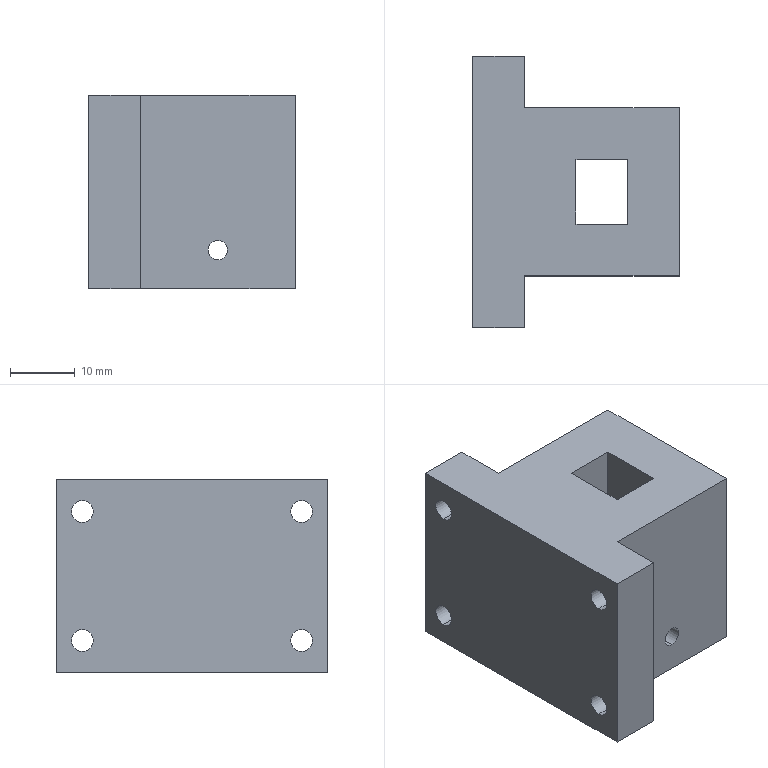Part | STEP file | X77b-01014 | 1 solid | 41 faces | box 32 x 42 x 30 mm | volume 25333 mm3 | cylinder 22 | plane 19 | commonest cylinder face diameters 3.4 x8 6 x8 3 x4 8 x2
STEP:
#1=CARTESIAN_POINT('',(-15.4,-53.814,28.));
#2=VERTEX_POINT('',#1);
#3=CARTESIAN_POINT('',(-15.4,-53.814,22.));
#4=VERTEX_POINT('',#3);
#5=CARTESIAN_POINT('',(-15.4,-53.814,25.));
#6=DIRECTION('',(1.,0.,0.));
#7=DIRECTION('',(0.,0.,-1.));
#8=AXIS2_PLACEMENT_3D('',#5,#6,#7);
#9=CIRCLE('',#8,3.);
#10=EDGE_CURVE('',#2,#4,#9,.T.);
#11=ORIENTED_EDGE('',*,*,#10,.F.);
#12=CARTESIAN_POINT('',(-12.,-53.814,28.));
#13=VERTEX_POINT('',#12);
#14=CARTESIAN_POINT('',(-12.,-53.814,28.));
#15=DIRECTION('',(1.,0.,0.));
#16=VECTOR('',#15,1000.);
#17=LINE('',#14,#16);
#18=EDGE_CURVE('',#2,#13,#17,.T.);
#19=ORIENTED_EDGE('',*,*,#18,.T.);
#20=CARTESIAN_POINT('',(-12.,-53.814,22.));
#21=VERTEX_POINT('',#20);
#22=CARTESIAN_POINT('',(-12.,-53.814,25.));
#23=DIRECTION('',(1.,0.,0.));
#24=DIRECTION('',(0.,0.,-1.));
#25=AXIS2_PLACEMENT_3D('',#22,#23,#24);
#26=CIRCLE('',#25,3.);
#27=EDGE_CURVE('',#13,#21,#26,.T.);
#28=ORIENTED_EDGE('',*,*,#27,.T.);
#29=CARTESIAN_POINT('',(-12.,-53.814,22.));
#30=DIRECTION('',(1.,0.,0.));
#31=VECTOR('',#30,1000.);
#32=LINE('',#29,#31);
#33=EDGE_CURVE('',#4,#21,#32,.T.);
#34=ORIENTED_EDGE('',*,*,#33,.F.);
#35=EDGE_LOOP('',(#11,#19,#28,#34));
#36=FACE_OUTER_BOUND('',#35,.T.);
#37=CARTESIAN_POINT('',(-12.,-53.814,25.));
#38=DIRECTION('',(1.,0.,0.));
#39=DIRECTION('',(0.,0.,-1.));
#40=AXIS2_PLACEMENT_3D('',#37,#38,#39);
#41=CYLINDRICAL_SURFACE('',#40,3.);
#42=ADVANCED_FACE('',(#36),#41,.F.);
#43=CARTESIAN_POINT('',(-20.,-53.814,26.7));
#44=VERTEX_POINT('',#43);
#45=CARTESIAN_POINT('',(-20.,-53.814,23.3));
#46=VERTEX_POINT('',#45);
#47=CARTESIAN_POINT('',(-20.,-53.814,25.));
#48=DIRECTION('',(1.,0.,0.));
#49=DIRECTION('',(0.,0.,-1.));
#50=AXIS2_PLACEMENT_3D('',#47,#48,#49);
#51=CIRCLE('',#50,1.7);
#52=EDGE_CURVE('',#44,#46,#51,.T.);
#53=ORIENTED_EDGE('',*,*,#52,.F.);
#54=CARTESIAN_POINT('',(-15.4,-53.814,26.7));
#55=VERTEX_POINT('',#54);
#56=CARTESIAN_POINT('',(-12.,-53.814,26.7));
#57=DIRECTION('',(1.,0.,0.));
#58=VECTOR('',#57,1000.);
#59=LINE('',#56,#58);
#60=EDGE_CURVE('',#44,#55,#59,.T.);
#61=ORIENTED_EDGE('',*,*,#60,.T.);
#62=CARTESIAN_POINT('',(-15.4,-53.814,23.3));
#63=VERTEX_POINT('',#62);
#64=CARTESIAN_POINT('',(-15.4,-53.814,25.));
#65=DIRECTION('',(1.,0.,0.));
#66=DIRECTION('',(0.,0.,-1.));
#67=AXIS2_PLACEMENT_3D('',#64,#65,#66);
#68=CIRCLE('',#67,1.7);
#69=EDGE_CURVE('',#55,#63,#68,.T.);
#70=ORIENTED_EDGE('',*,*,#69,.T.);
#71=CARTESIAN_POINT('',(-12.,-53.814,23.3));
#72=DIRECTION('',(1.,0.,0.));
#73=VECTOR('',#72,1000.);
#74=LINE('',#71,#73);
#75=EDGE_CURVE('',#46,#63,#74,.T.);
#76=ORIENTED_EDGE('',*,*,#75,.F.);
#77=EDGE_LOOP('',(#53,#61,#70,#76));
#78=FACE_OUTER_BOUND('',#77,.T.);
#79=CARTESIAN_POINT('',(-12.,-53.814,25.));
#80=DIRECTION('',(1.,0.,0.));
#81=DIRECTION('',(0.,0.,-1.));
#82=AXIS2_PLACEMENT_3D('',#79,#80,#81);
#83=CYLINDRICAL_SURFACE('',#82,1.7);
#84=ADVANCED_FACE('',(#78),#83,.F.);
#85=CARTESIAN_POINT('',(-15.4,-53.814,8.));
#86=VERTEX_POINT('',#85);
#87=CARTESIAN_POINT('',(-15.4,-53.814,2.));
#88=VERTEX_POINT('',#87);
#89=CARTESIAN_POINT('',(-15.4,-53.814,5.));
#90=DIRECTION('',(1.,0.,0.));
#91=DIRECTION('',(0.,0.,-1.));
#92=AXIS2_PLACEMENT_3D('',#89,#90,#91);
#93=CIRCLE('',#92,3.);
#94=EDGE_CURVE('',#86,#88,#93,.T.);
#95=ORIENTED_EDGE('',*,*,#94,.F.);
#96=CARTESIAN_POINT('',(-12.,-53.814,8.));
#97=VERTEX_POINT('',#96);
#98=CARTESIAN_POINT('',(-12.,-53.814,8.));
#99=DIRECTION('',(1.,0.,0.));
#100=VECTOR('',#99,1000.);
#101=LINE('',#98,#100);
#102=EDGE_CURVE('',#86,#97,#101,.T.);
#103=ORIENTED_EDGE('',*,*,#102,.T.);
#104=CARTESIAN_POINT('',(-12.,-53.814,2.));
#105=VERTEX_POINT('',#104);
#106=CARTESIAN_POINT('',(-12.,-53.814,5.));
#107=DIRECTION('',(1.,0.,0.));
#108=DIRECTION('',(0.,0.,-1.));
#109=AXIS2_PLACEMENT_3D('',#106,#107,#108);
#110=CIRCLE('',#109,3.);
#111=EDGE_CURVE('',#97,#105,#110,.T.);
#112=ORIENTED_EDGE('',*,*,#111,.T.);
#113=CARTESIAN_POINT('',(-12.,-53.814,2.));
#114=DIRECTION('',(1.,0.,0.));
#115=VECTOR('',#114,1000.);
#116=LINE('',#113,#115);
#117=EDGE_CURVE('',#88,#105,#116,.T.);
#118=ORIENTED_EDGE('',*,*,#117,.F.);
#119=EDGE_LOOP('',(#95,#103,#112,#118));
#120=FACE_OUTER_BOUND('',#119,.T.);
#121=CARTESIAN_POINT('',(-12.,-53.814,5.));
#122=DIRECTION('',(1.,0.,0.));
#123=DIRECTION('',(0.,0.,-1.));
#124=AXIS2_PLACEMENT_3D('',#121,#122,#123);
#125=CYLINDRICAL_SURFACE('',#124,3.);
#126=ADVANCED_FACE('',(#120),#125,.F.);
#127=CARTESIAN_POINT('',(-20.,-53.814,6.7));
#128=VERTEX_POINT('',#127);
#129=CARTESIAN_POINT('',(-20.,-53.814,3.3));
#130=VERTEX_POINT('',#129);
#131=CARTESIAN_POINT('',(-20.,-53.814,5.));
#132=DIRECTION('',(1.,0.,0.));
#133=DIRECTION('',(0.,0.,-1.));
#134=AXIS2_PLACEMENT_3D('',#131,#132,#133);
#135=CIRCLE('',#134,1.7);
#136=EDGE_CURVE('',#128,#130,#135,.T.);
#137=ORIENTED_EDGE('',*,*,#136,.F.);
#138=CARTESIAN_POINT('',(-15.4,-53.814,6.7));
#139=VERTEX_POINT('',#138);
#140=CARTESIAN_POINT('',(-12.,-53.814,6.7));
#141=DIRECTION('',(1.,0.,0.));
#142=VECTOR('',#141,1000.);
#143=LINE('',#140,#142);
#144=EDGE_CURVE('',#128,#139,#143,.T.);
#145=ORIENTED_EDGE('',*,*,#144,.T.);
#146=CARTESIAN_POINT('',(-15.4,-53.814,3.3));
#147=VERTEX_POINT('',#146);
#148=CARTESIAN_POINT('',(-15.4,-53.814,5.));
#149=DIRECTION('',(1.,0.,0.));
#150=DIRECTION('',(0.,0.,-1.));
#151=AXIS2_PLACEMENT_3D('',#148,#149,#150);
#152=CIRCLE('',#151,1.7);
#153=EDGE_CURVE('',#139,#147,#152,.T.);
#154=ORIENTED_EDGE('',*,*,#153,.T.);
#155=CARTESIAN_POINT('',(-12.,-53.814,3.3));
#156=DIRECTION('',(1.,0.,0.));
#157=VECTOR('',#156,1000.);
#158=LINE('',#155,#157);
#159=EDGE_CURVE('',#130,#147,#158,.T.);
#160=ORIENTED_EDGE('',*,*,#159,.F.);
#161=EDGE_LOOP('',(#137,#145,#154,#160));
#162=FACE_OUTER_BOUND('',#161,.T.);
#163=CARTESIAN_POINT('',(-12.,-53.814,5.));
#164=DIRECTION('',(1.,0.,0.));
#165=DIRECTION('',(0.,0.,-1.));
#166=AXIS2_PLACEMENT_3D('',#163,#164,#165);
#167=CYLINDRICAL_SURFACE('',#166,1.7);
#168=ADVANCED_FACE('',(#162),#167,.F.);
#169=CARTESIAN_POINT('',(-15.4,-87.814,28.));
#170=VERTEX_POINT('',#169);
#171=CARTESIAN_POINT('',(-15.4,-87.814,22.));
#172=VERTEX_POINT('',#171);
#173=CARTESIAN_POINT('',(-15.4,-87.814,25.));
#174=DIRECTION('',(1.,0.,0.));
#175=DIRECTION('',(0.,0.,-1.));
#176=AXIS2_PLACEMENT_3D('',#173,#174,#175);
#177=CIRCLE('',#176,3.);
#178=EDGE_CURVE('',#170,#172,#177,.T.);
#179=ORIENTED_EDGE('',*,*,#178,.F.);
#180=CARTESIAN_POINT('',(-12.,-87.814,28.));
#181=VERTEX_POINT('',#180);
#182=CARTESIAN_POINT('',(-12.,-87.814,28.));
#183=DIRECTION('',(1.,0.,0.));
#184=VECTOR('',#183,1000.);
#185=LINE('',#182,#184);
#186=EDGE_CURVE('',#170,#181,#185,.T.);
#187=ORIENTED_EDGE('',*,*,#186,.T.);
#188=CARTESIAN_POINT('',(-12.,-87.814,22.));
#189=VERTEX_POINT('',#188);
#190=CARTESIAN_POINT('',(-12.,-87.814,25.));
#191=DIRECTION('',(1.,0.,0.));
#192=DIRECTION('',(0.,0.,-1.));
#193=AXIS2_PLACEMENT_3D('',#190,#191,#192);
#194=CIRCLE('',#193,3.);
#195=EDGE_CURVE('',#181,#189,#194,.T.);
#196=ORIENTED_EDGE('',*,*,#195,.T.);
#197=CARTESIAN_POINT('',(-12.,-87.814,22.));
#198=DIRECTION('',(1.,0.,0.));
#199=VECTOR('',#198,1000.);
#200=LINE('',#197,#199);
#201=EDGE_CURVE('',#172,#189,#200,.T.);
#202=ORIENTED_EDGE('',*,*,#201,.F.);
#203=EDGE_LOOP('',(#179,#187,#196,#202));
#204=FACE_OUTER_BOUND('',#203,.T.);
#205=CARTESIAN_POINT('',(-12.,-87.814,25.));
#206=DIRECTION('',(1.,0.,0.));
#207=DIRECTION('',(0.,0.,-1.));
#208=AXIS2_PLACEMENT_3D('',#205,#206,#207);
#209=CYLINDRICAL_SURFACE('',#208,3.);
#210=ADVANCED_FACE('',(#204),#209,.F.);
#211=CARTESIAN_POINT('',(-20.,-87.814,26.7));
#212=VERTEX_POINT('',#211);
#213=CARTESIAN_POINT('',(-20.,-87.814,23.3));
#214=VERTEX_POINT('',#213);
#215=CARTESIAN_POINT('',(-20.,-87.814,25.));
#216=DIRECTION('',(1.,0.,0.));
#217=DIRECTION('',(0.,0.,-1.));
#218=AXIS2_PLACEMENT_3D('',#215,#216,#217);
#219=CIRCLE('',#218,1.7);
#220=EDGE_CURVE('',#212,#214,#219,.T.);
#221=ORIENTED_EDGE('',*,*,#220,.F.);
#222=CARTESIAN_POINT('',(-15.4,-87.814,26.7));
#223=VERTEX_POINT('',#222);
#224=CARTESIAN_POINT('',(-12.,-87.814,26.7));
#225=DIRECTION('',(1.,0.,0.));
#226=VECTOR('',#225,1000.);
#227=LINE('',#224,#226);
#228=EDGE_CURVE('',#212,#223,#227,.T.);
#229=ORIENTED_EDGE('',*,*,#228,.T.);
#230=CARTESIAN_POINT('',(-15.4,-87.814,23.3));
#231=VERTEX_POINT('',#230);
#232=CARTESIAN_POINT('',(-15.4,-87.814,25.));
#233=DIRECTION('',(1.,0.,0.));
#234=DIRECTION('',(0.,0.,-1.));
#235=AXIS2_PLACEMENT_3D('',#232,#233,#234);
#236=CIRCLE('',#235,1.7);
#237=EDGE_CURVE('',#223,#231,#236,.T.);
#238=ORIENTED_EDGE('',*,*,#237,.T.);
#239=CARTESIAN_POINT('',(-12.,-87.814,23.3));
#240=DIRECTION('',(1.,0.,0.));
#241=VECTOR('',#240,1000.);
#242=LINE('',#239,#241);
#243=EDGE_CURVE('',#214,#231,#242,.T.);
#244=ORIENTED_EDGE('',*,*,#243,.F.);
#245=EDGE_LOOP('',(#221,#229,#238,#244));
#246=FACE_OUTER_BOUND('',#245,.T.);
#247=CARTESIAN_POINT('',(-12.,-87.814,25.));
#248=DIRECTION('',(1.,0.,0.));
#249=DIRECTION('',(0.,0.,-1.));
#250=AXIS2_PLACEMENT_3D('',#247,#248,#249);
#251=CYLINDRICAL_SURFACE('',#250,1.7);
#252=ADVANCED_FACE('',(#246),#251,.F.);
#253=CARTESIAN_POINT('',(-15.4,-87.814,8.));
#254=VERTEX_POINT('',#253);
#255=CARTESIAN_POINT('',(-15.4,-87.814,2.));
#256=VERTEX_POINT('',#255);
#257=CARTESIAN_POINT('',(-15.4,-87.814,5.));
#258=DIRECTION('',(1.,0.,0.));
#259=DIRECTION('',(0.,0.,-1.));
#260=AXIS2_PLACEMENT_3D('',#257,#258,#259);
#261=CIRCLE('',#260,3.);
#262=EDGE_CURVE('',#254,#256,#261,.T.);
#263=ORIENTED_EDGE('',*,*,#262,.F.);
#264=CARTESIAN_POINT('',(-12.,-87.814,8.));
#265=VERTEX_POINT('',#264);
#266=CARTESIAN_POINT('',(-12.,-87.814,8.));
#267=DIRECTION('',(1.,0.,0.));
#268=VECTOR('',#267,1000.);
#269=LINE('',#266,#268);
#270=EDGE_CURVE('',#254,#265,#269,.T.);
#271=ORIENTED_EDGE('',*,*,#270,.T.);
#272=CARTESIAN_POINT('',(-12.,-87.814,2.));
#273=VERTEX_POINT('',#272);
#274=CARTESIAN_POINT('',(-12.,-87.814,5.));
#275=DIRECTION('',(1.,0.,0.));
#276=DIRECTION('',(0.,0.,-1.));
#277=AXIS2_PLACEMENT_3D('',#274,#275,#276);
#278=CIRCLE('',#277,3.);
#279=EDGE_CURVE('',#265,#273,#278,.T.);
#280=ORIENTED_EDGE('',*,*,#279,.T.);
#281=CARTESIAN_POINT('',(-12.,-87.814,2.));
#282=DIRECTION('',(1.,0.,0.));
#283=VECTOR('',#282,1000.);
#284=LINE('',#281,#283);
#285=EDGE_CURVE('',#256,#273,#284,.T.);
#286=ORIENTED_EDGE('',*,*,#285,.F.);
#287=EDGE_LOOP('',(#263,#271,#280,#286));
#288=FACE_OUTER_BOUND('',#287,.T.);
#289=CARTESIAN_POINT('',(-12.,-87.814,5.));
#290=DIRECTION('',(1.,0.,0.));
#291=DIRECTION('',(0.,0.,-1.));
#292=AXIS2_PLACEMENT_3D('',#289,#290,#291);
#293=CYLINDRICAL_SURFACE('',#292,3.);
#294=ADVANCED_FACE('',(#288),#293,.F.);
#295=CARTESIAN_POINT('',(-20.,-87.814,6.7));
#296=VERTEX_POINT('',#295);
#297=CARTESIAN_POINT('',(-20.,-87.814,3.3));
#298=VERTEX_POINT('',#297);
#299=CARTESIAN_POINT('',(-20.,-87.814,5.));
#300=DIRECTION('',(1.,0.,0.));
#301=DIRECTION('',(0.,0.,-1.));
#302=AXIS2_PLACEMENT_3D('',#299,#300,#301);
#303=CIRCLE('',#302,1.7);
#304=EDGE_CURVE('',#296,#298,#303,.T.);
#305=ORIENTED_EDGE('',*,*,#304,.F.);
#306=CARTESIAN_POINT('',(-15.4,-87.814,6.7));
#307=VERTEX_POINT('',#306);
#308=CARTESIAN_POINT('',(-12.,-87.814,6.7));
#309=DIRECTION('',(1.,0.,0.));
#310=VECTOR('',#309,1000.);
#311=LINE('',#308,#310);
#312=EDGE_CURVE('',#296,#307,#311,.T.);
#313=ORIENTED_EDGE('',*,*,#312,.T.);
#314=CARTESIAN_POINT('',(-15.4,-87.814,3.3));
#315=VERTEX_POINT('',#314);
#316=CARTESIAN_POINT('',(-15.4,-87.814,5.));
#317=DIRECTION('',(1.,0.,0.));
#318=DIRECTION('',(0.,0.,-1.));
#319=AXIS2_PLACEMENT_3D('',#316,#317,#318);
#320=CIRCLE('',#319,1.7);
#321=EDGE_CURVE('',#307,#315,#320,.T.);
#322=ORIENTED_EDGE('',*,*,#321,.T.);
#323=CARTESIAN_POINT('',(-12.,-87.814,3.3));
#324=DIRECTION('',(1.,0.,0.));
#325=VECTOR('',#324,1000.);
#326=LINE('',#323,#325);
#327=EDGE_CURVE('',#298,#315,#326,.T.);
#328=ORIENTED_EDGE('',*,*,#327,.F.);
#329=EDGE_LOOP('',(#305,#313,#322,#328));
#330=FACE_OUTER_BOUND('',#329,.T.);
#331=CARTESIAN_POINT('',(-12.,-87.814,5.));
#332=DIRECTION('',(1.,0.,0.));
#333=DIRECTION('',(0.,0.,-1.));
#334=AXIS2_PLACEMENT_3D('',#331,#332,#333);
#335=CYLINDRICAL_SURFACE('',#334,1.7);
#336=ADVANCED_FACE('',(#330),#335,.F.);
#337=CARTESIAN_POINT('',(0.,-83.814,4.5));
#338=VERTEX_POINT('',#337);
#339=CARTESIAN_POINT('',(0.,-83.814,7.5));
#340=VERTEX_POINT('',#339);
#341=CARTESIAN_POINT('',(0.,-83.814,6.));
#342=DIRECTION('',(0.,1.,0.));
#343=DIRECTION('',(0.,0.,1.));
#344=AXIS2_PLACEMENT_3D('',#341,#342,#343);
#345=CIRCLE('',#344,1.5);
#346=EDGE_CURVE('',#338,#340,#345,.T.);
#347=ORIENTED_EDGE('',*,*,#346,.F.);
#348=CARTESIAN_POINT('',(0.,-75.814,4.5));
#349=VERTEX_POINT('',#348);
#350=CARTESIAN_POINT('',(0.,-57.814,4.5));
#351=DIRECTION('',(0.,1.,0.));
#352=VECTOR('',#351,1000.);
#353=LINE('',#350,#352);
#354=EDGE_CURVE('',#338,#349,#353,.T.);
#355=ORIENTED_EDGE('',*,*,#354,.T.);
#356=CARTESIAN_POINT('',(0.,-75.814,7.5));
#357=VERTEX_POINT('',#356);
#358=CARTESIAN_POINT('',(0.,-75.814,6.));
#359=DIRECTION('',(0.,1.,0.));
#360=DIRECTION('',(0.,0.,1.));
#361=AXIS2_PLACEMENT_3D('',#358,#359,#360);
#362=CIRCLE('',#361,1.5);
#363=EDGE_CURVE('',#349,#357,#362,.T.);
#364=ORIENTED_EDGE('',*,*,#363,.T.);
#365=CARTESIAN_POINT('',(0.,-57.814,7.5));
#366=DIRECTION('',(0.,1.,0.));
#367=VECTOR('',#366,1000.);
#368=LINE('',#365,#367);
#369=EDGE_CURVE('',#340,#357,#368,.T.);
#370=ORIENTED_EDGE('',*,*,#369,.F.);
#371=EDGE_LOOP('',(#347,#355,#364,#370));
#372=FACE_OUTER_BOUND('',#371,.T.);
#373=CARTESIAN_POINT('',(0.,-57.814,6.));
#374=DIRECTION('',(0.,1.,0.));
#375=DIRECTION('',(0.,0.,1.));
#376=AXIS2_PLACEMENT_3D('',#373,#374,#375);
#377=CYLINDRICAL_SURFACE('',#376,1.5);
#378=ADVANCED_FACE('',(#372),#377,.F.);
#379=CARTESIAN_POINT('',(0.,-65.814,7.5));
#380=VERTEX_POINT('',#379);
#381=CARTESIAN_POINT('',(0.,-65.814,4.5));
#382=VERTEX_POINT('',#381);
#383=CARTESIAN_POINT('',(0.,-65.814,6.));
#384=DIRECTION('',(0.,-1.,0.));
#385=DIRECTION('',(0.,0.,-1.));
#386=AXIS2_PLACEMENT_3D('',#383,#384,#385);
#387=CIRCLE('',#386,1.5);
#388=EDGE_CURVE('',#380,#382,#387,.T.);
#389=ORIENTED_EDGE('',*,*,#388,.T.);
#390=CARTESIAN_POINT('',(0.,-57.814,4.5));
#391=VERTEX_POINT('',#390);
#392=CARTESIAN_POINT('',(0.,-57.814,4.5));
#393=DIRECTION('',(0.,1.,0.));
#394=VECTOR('',#393,1000.);
#395=LINE('',#392,#394);
#396=EDGE_CURVE('',#382,#391,#395,.T.);
#397=ORIENTED_EDGE('',*,*,#396,.T.);
#398=CARTESIAN_POINT('',(0.,-57.814,7.5));
#399=VERTEX_POINT('',#398);
#400=CARTESIAN_POINT('',(0.,-57.814,6.));
#401=DIRECTION('',(0.,1.,0.));
#402=DIRECTION('',(0.,0.,1.));
#403=AXIS2_PLACEMENT_3D('',#400,#401,#402);
#404=CIRCLE('',#403,1.5);
#405=EDGE_CURVE('',#391,#399,#404,.T.);
#406=ORIENTED_EDGE('',*,*,#405,.T.);
#407=CARTESIAN_POINT('',(0.,-57.814,7.5));
#408=DIRECTION('',(0.,1.,0.));
#409=VECTOR('',#408,1000.);
#410=LINE('',#407,#409);
#411=EDGE_CURVE('',#380,#399,#410,.T.);
#412=ORIENTED_EDGE('',*,*,#411,.F.);
#413=EDGE_LOOP('',(#389,#397,#406,#412));
#414=FACE_OUTER_BOUND('',#413,.T.);
#415=CARTESIAN_POINT('',(0.,-57.814,6.));
#416=DIRECTION('',(0.,1.,0.));
#417=DIRECTION('',(0.,0.,1.));
#418=AXIS2_PLACEMENT_3D('',#415,#416,#417);
#419=CYLINDRICAL_SURFACE('',#418,1.5);
#420=ADVANCED_FACE('',(#414),#419,.F.);
#421=CARTESIAN_POINT('',(-4.,-65.815,15.));
#422=VERTEX_POINT('',#421);
#423=CARTESIAN_POINT('',(0.,-65.814,11.));
#424=VERTEX_POINT('',#423);
#425=CARTESIAN_POINT('',(0.,-65.814,15.));
#426=DIRECTION('',(0.,-1.,0.));
#427=DIRECTION('',(0.,0.,-1.));
#428=AXIS2_PLACEMENT_3D('',#425,#426,#427);
#429=CIRCLE('',#428,4.);
#430=EDGE_CURVE('',#422,#424,#429,.T.);
#431=ORIENTED_EDGE('',*,*,#430,.T.);
#432=CARTESIAN_POINT('',(0.,-57.814,11.));
#433=VERTEX_POINT('',#432);
#434=CARTESIAN_POINT('',(0.,-57.814,11.));
#435=DIRECTION('',(0.,1.,0.));
#436=VECTOR('',#435,1000.);
#437=LINE('',#434,#436);
#438=EDGE_CURVE('',#424,#433,#437,.T.);
#439=ORIENTED_EDGE('',*,*,#438,.T.);
#440=CARTESIAN_POINT('',(0.,-57.814,19.));
#441=VERTEX_POINT('',#440);
#442=CARTESIAN_POINT('',(0.,-57.814,15.));
#443=DIRECTION('',(0.,1.,0.));
#444=DIRECTION('',(0.,0.,1.));
#445=AXIS2_PLACEMENT_3D('',#442,#443,#444);
#446=CIRCLE('',#445,4.);
#447=EDGE_CURVE('',#433,#441,#446,.T.);
#448=ORIENTED_EDGE('',*,*,#447,.T.);
#449=CARTESIAN_POINT('',(0.,-65.814,19.));
#450=VERTEX_POINT('',#449);
#451=CARTESIAN_POINT('',(0.,-57.814,19.));
#452=DIRECTION('',(0.,1.,0.));
#453=VECTOR('',#452,1000.);
#454=LINE('',#451,#453);
#455=EDGE_CURVE('',#450,#441,#454,.T.);
#456=ORIENTED_EDGE('',*,*,#455,.F.);
#457=CARTESIAN_POINT('',(0.,-65.814,15.));
#458=DIRECTION('',(0.,-1.,0.));
#459=DIRECTION('',(0.,0.,-1.));
#460=AXIS2_PLACEMENT_3D('',#457,#458,#459);
#461=CIRCLE('',#460,4.);
#462=EDGE_CURVE('',#450,#422,#461,.T.);
#463=ORIENTED_EDGE('',*,*,#462,.T.);
#464=EDGE_LOOP('',(#431,#439,#448,#456,#463));
#465=FACE_OUTER_BOUND('',#464,.T.);
#466=CARTESIAN_POINT('',(0.,-57.814,15.));
#467=DIRECTION('',(0.,1.,0.));
#468=DIRECTION('',(0.,0.,1.));
#469=AXIS2_PLACEMENT_3D('',#466,#467,#468);
#470=CYLINDRICAL_SURFACE('',#469,4.);
#471=ADVANCED_FACE('',(#465),#470,.F.);
#472=CARTESIAN_POINT('',(4.,-65.815,15.));
#473=VERTEX_POINT('',#472);
#474=CARTESIAN_POINT('',(0.,-65.814,15.));
#475=DIRECTION('',(0.,-1.,0.));
#476=DIRECTION('',(0.,0.,-1.));
#477=AXIS2_PLACEMENT_3D('',#474,#475,#476);
#478=CIRCLE('',#477,4.);
#479=EDGE_CURVE('',#473,#450,#478,.T.);
#480=ORIENTED_EDGE('',*,*,#479,.F.);
#481=CARTESIAN_POINT('',(4.,-65.814,30.));
#482=VERTEX_POINT('',#481);
#483=CARTESIAN_POINT('',(4.,-65.814,30.));
#484=DIRECTION('',(0.,0.,-1.));
#485=VECTOR('',#484,1000.);
#486=LINE('',#483,#485);
#487=EDGE_CURVE('',#482,#473,#486,.T.);
#488=ORIENTED_EDGE('',*,*,#487,.F.);
#489=CARTESIAN_POINT('',(-4.,-65.814,30.));
#490=VERTEX_POINT('',#489);
#491=CARTESIAN_POINT('',(-4.,-65.814,30.));
#492=DIRECTION('',(-1.,0.,0.));
#493=VECTOR('',#492,1000.);
#494=LINE('',#491,#493);
#495=EDGE_CURVE('',#482,#490,#494,.T.);
#496=ORIENTED_EDGE('',*,*,#495,.T.);
#497=CARTESIAN_POINT('',(-4.,-65.814,30.));
#498=DIRECTION('',(0.,0.,-1.));
#499=VECTOR('',#498,1000.);
#500=LINE('',#497,#499);
#501=EDGE_CURVE('',#490,#422,#500,.T.);
#502=ORIENTED_EDGE('',*,*,#501,.T.);
#503=ORIENTED_EDGE('',*,*,#462,.F.);
#504=EDGE_LOOP('',(#480,#488,#496,#502,#503));
#505=FACE_OUTER_BOUND('',#504,.T.);
#506=CARTESIAN_POINT('',(-4.,-65.814,30.));
#507=DIRECTION('',(0.,-1.,0.));
#508=DIRECTION('',(0.,0.,-1.));
#509=AXIS2_PLACEMENT_3D('',#506,#507,#508);
#510=PLANE('',#509);
#511=ADVANCED_FACE('',(#505),#510,.T.);
#512=CARTESIAN_POINT('',(12.,-57.814,30.));
#513=VERTEX_POINT('',#512);
#514=CARTESIAN_POINT('',(-12.,-57.814,30.));
#515=VERTEX_POINT('',#514);
#516=CARTESIAN_POINT('',(-12.,-57.814,30.));
#517=DIRECTION('',(-1.,0.,0.));
#518=VECTOR('',#517,1000.);
#519=LINE('',#516,#518);
#520=EDGE_CURVE('',#513,#515,#519,.T.);
#521=ORIENTED_EDGE('',*,*,#520,.T.);
#522=CARTESIAN_POINT('',(-12.,-49.814,30.));
#523=VERTEX_POINT('',#522);
#524=CARTESIAN_POINT('',(-12.,-91.814,30.));
#525=DIRECTION('',(0.,1.,0.));
#526=VECTOR('',#525,1000.);
#527=LINE('',#524,#526);
#528=EDGE_CURVE('',#515,#523,#527,.T.);
#529=ORIENTED_EDGE('',*,*,#528,.T.);
#530=CARTESIAN_POINT('',(-20.,-49.814,30.));
#531=VERTEX_POINT('',#530);
#532=CARTESIAN_POINT('',(-12.,-49.814,30.));
#533=DIRECTION('',(1.,0.,0.));
#534=VECTOR('',#533,1000.);
#535=LINE('',#532,#534);
#536=EDGE_CURVE('',#531,#523,#535,.T.);
#537=ORIENTED_EDGE('',*,*,#536,.F.);
#538=CARTESIAN_POINT('',(-20.,-91.814,30.));
#539=VERTEX_POINT('',#538);
#540=CARTESIAN_POINT('',(-20.,-91.814,30.));
#541=DIRECTION('',(0.,1.,0.));
#542=VECTOR('',#541,1000.);
#543=LINE('',#540,#542);
#544=EDGE_CURVE('',#539,#531,#543,.T.);
#545=ORIENTED_EDGE('',*,*,#544,.F.);
#546=CARTESIAN_POINT('',(-12.,-91.814,30.));
#547=VERTEX_POINT('',#546);
#548=CARTESIAN_POINT('',(-12.,-91.814,30.));
#549=DIRECTION('',(1.,0.,0.));
#550=VECTOR('',#549,1000.);
#551=LINE('',#548,#550);
#552=EDGE_CURVE('',#539,#547,#551,.T.);
#553=ORIENTED_EDGE('',*,*,#552,.T.);
#554=CARTESIAN_POINT('',(-12.,-83.814,30.));
#555=VERTEX_POINT('',#554);
#556=CARTESIAN_POINT('',(-12.,-91.814,30.));
#557=DIRECTION('',(0.,1.,0.));
#558=VECTOR('',#557,1000.);
#559=LINE('',#556,#558);
#560=EDGE_CURVE('',#547,#555,#559,.T.);
#561=ORIENTED_EDGE('',*,*,#560,.T.);
#562=CARTESIAN_POINT('',(12.,-83.814,30.));
#563=VERTEX_POINT('',#562);
#564=CARTESIAN_POINT('',(-12.,-83.814,30.));
#565=DIRECTION('',(1.,0.,0.));
#566=VECTOR('',#565,1000.);
#567=LINE('',#564,#566);
#568=EDGE_CURVE('',#555,#563,#567,.T.);
#569=ORIENTED_EDGE('',*,*,#568,.T.);
#570=CARTESIAN_POINT('',(12.,-83.814,30.));
#571=DIRECTION('',(0.,1.,0.));
#572=VECTOR('',#571,1000.);
#573=LINE('',#570,#572);
#574=EDGE_CURVE('',#563,#513,#573,.T.);
#575=ORIENTED_EDGE('',*,*,#574,.T.);
#576=EDGE_LOOP('',(#521,#529,#537,#545,#553,#561,#569,#575));
#577=FACE_OUTER_BOUND('',#576,.T.);
#578=CARTESIAN_POINT('',(-4.,-75.814,30.));
#579=VERTEX_POINT('',#578);
#580=CARTESIAN_POINT('',(-4.,-75.814,30.));
#581=DIRECTION('',(0.,-1.,0.));
#582=VECTOR('',#581,1000.);
#583=LINE('',#580,#582);
#584=EDGE_CURVE('',#490,#579,#583,.T.);
#585=ORIENTED_EDGE('',*,*,#584,.F.);
#586=ORIENTED_EDGE('',*,*,#495,.F.);
#587=CARTESIAN_POINT('',(4.,-75.814,30.));
#588=VERTEX_POINT('',#587);
#589=CARTESIAN_POINT('',(4.,-75.814,30.));
#590=DIRECTION('',(0.,1.,0.));
#591=VECTOR('',#590,1000.);
#592=LINE('',#589,#591);
#593=EDGE_CURVE('',#588,#482,#592,.T.);
#594=ORIENTED_EDGE('',*,*,#593,.F.);
#595=CARTESIAN_POINT('',(-4.,-75.814,30.));
#596=DIRECTION('',(1.,0.,0.));
#597=VECTOR('',#596,1000.);
#598=LINE('',#595,#597);
#599=EDGE_CURVE('',#579,#588,#598,.T.);
#600=ORIENTED_EDGE('',*,*,#599,.F.);
#601=EDGE_LOOP('',(#585,#586,#594,#600));
#602=FACE_BOUND('',#601,.T.);
#603=CARTESIAN_POINT('',(-12.,-57.814,30.));
#604=DIRECTION('',(0.,0.,-1.));
#605=DIRECTION('',(-1.,0.,0.));
#606=AXIS2_PLACEMENT_3D('',#603,#604,#605);
#607=PLANE('',#606);
#608=ADVANCED_FACE('',(#577,#602),#607,.F.);
#609=CARTESIAN_POINT('',(-12.,-83.814,0.));
#610=VERTEX_POINT('',#609);
#611=CARTESIAN_POINT('',(12.,-83.814,0.));
#612=VERTEX_POINT('',#611);
#613=CARTESIAN_POINT('',(-12.,-83.814,0.));
#614=DIRECTION('',(1.,0.,0.));
#615=VECTOR('',#614,1000.);
#616=LINE('',#613,#615);
#617=EDGE_CURVE('',#610,#612,#616,.T.);
#618=ORIENTED_EDGE('',*,*,#617,.F.);
#619=CARTESIAN_POINT('',(-12.,-91.814,0.));
#620=VERTEX_POINT('',#619);
#621=CARTESIAN_POINT('',(-12.,-91.814,0.));
#622=DIRECTION('',(0.,1.,0.));
#623=VECTOR('',#622,1000.);
#624=LINE('',#621,#623);
#625=EDGE_CURVE('',#620,#610,#624,.T.);
#626=ORIENTED_EDGE('',*,*,#625,.F.);
#627=CARTESIAN_POINT('',(-20.,-91.814,0.));
#628=VERTEX_POINT('',#627);
#629=CARTESIAN_POINT('',(-12.,-91.814,0.));
#630=DIRECTION('',(-1.,0.,0.));
#631=VECTOR('',#630,1000.);
#632=LINE('',#629,#631);
#633=EDGE_CURVE('',#620,#628,#632,.T.);
#634=ORIENTED_EDGE('',*,*,#633,.T.);
#635=CARTESIAN_POINT('',(-20.,-49.814,0.));
#636=VERTEX_POINT('',#635);
#637=CARTESIAN_POINT('',(-20.,-91.814,0.));
#638=DIRECTION('',(0.,1.,0.));
#639=VECTOR('',#638,1000.);
#640=LINE('',#637,#639);
#641=EDGE_CURVE('',#628,#636,#640,.T.);
#642=ORIENTED_EDGE('',*,*,#641,.T.);
#643=CARTESIAN_POINT('',(-12.,-49.814,0.));
#644=VERTEX_POINT('',#643);
#645=CARTESIAN_POINT('',(-12.,-49.814,0.));
#646=DIRECTION('',(-1.,0.,0.));
#647=VECTOR('',#646,1000.);
#648=LINE('',#645,#647);
#649=EDGE_CURVE('',#644,#636,#648,.T.);
#650=ORIENTED_EDGE('',*,*,#649,.F.);
#651=CARTESIAN_POINT('',(-12.,-57.814,0.));
#652=VERTEX_POINT('',#651);
#653=CARTESIAN_POINT('',(-12.,-91.814,0.));
#654=DIRECTION('',(0.,1.,0.));
#655=VECTOR('',#654,1000.);
#656=LINE('',#653,#655);
#657=EDGE_CURVE('',#652,#644,#656,.T.);
#658=ORIENTED_EDGE('',*,*,#657,.F.);
#659=CARTESIAN_POINT('',(12.,-57.814,0.));
#660=VERTEX_POINT('',#659);
#661=CARTESIAN_POINT('',(-12.,-57.814,0.));
#662=DIRECTION('',(-1.,0.,0.));
#663=VECTOR('',#662,1000.);
#664=LINE('',#661,#663);
#665=EDGE_CURVE('',#660,#652,#664,.T.);
#666=ORIENTED_EDGE('',*,*,#665,.F.);
#667=CARTESIAN_POINT('',(12.,-83.814,0.));
#668=DIRECTION('',(0.,1.,0.));
#669=VECTOR('',#668,1000.);
#670=LINE('',#667,#669);
#671=EDGE_CURVE('',#612,#660,#670,.T.);
#672=ORIENTED_EDGE('',*,*,#671,.F.);
#673=EDGE_LOOP('',(#618,#626,#634,#642,#650,#658,#666,#672));
#674=FACE_OUTER_BOUND('',#673,.T.);
#675=CARTESIAN_POINT('',(4.,-65.814,0.));
#676=VERTEX_POINT('',#675);
#677=CARTESIAN_POINT('',(-4.,-65.814,0.));
#678=VERTEX_POINT('',#677);
#679=CARTESIAN_POINT('',(-4.,-65.814,0.));
#680=DIRECTION('',(-1.,0.,0.));
#681=VECTOR('',#680,1000.);
#682=LINE('',#679,#681);
#683=EDGE_CURVE('',#676,#678,#682,.T.);
#684=ORIENTED_EDGE('',*,*,#683,.T.);
#685=CARTESIAN_POINT('',(-4.,-75.814,0.));
#686=VERTEX_POINT('',#685);
#687=CARTESIAN_POINT('',(-4.,-75.814,0.));
#688=DIRECTION('',(0.,-1.,0.));
#689=VECTOR('',#688,1000.);
#690=LINE('',#687,#689);
#691=EDGE_CURVE('',#678,#686,#690,.T.);
#692=ORIENTED_EDGE('',*,*,#691,.T.);
#693=CARTESIAN_POINT('',(4.,-75.814,0.));
#694=VERTEX_POINT('',#693);
#695=CARTESIAN_POINT('',(-4.,-75.814,0.));
#696=DIRECTION('',(1.,0.,0.));
#697=VECTOR('',#696,1000.);
#698=LINE('',#695,#697);
#699=EDGE_CURVE('',#686,#694,#698,.T.);
#700=ORIENTED_EDGE('',*,*,#699,.T.);
#701=CARTESIAN_POINT('',(4.,-75.814,0.));
#702=DIRECTION('',(0.,1.,0.));
#703=VECTOR('',#702,1000.);
#704=LINE('',#701,#703);
#705=EDGE_CURVE('',#694,#676,#704,.T.);
#706=ORIENTED_EDGE('',*,*,#705,.T.);
#707=EDGE_LOOP('',(#684,#692,#700,#706));
#708=FACE_BOUND('',#707,.T.);
#709=CARTESIAN_POINT('',(-12.,-57.814,0.));
#710=DIRECTION('',(0.,0.,-1.));
#711=DIRECTION('',(-1.,0.,0.));
#712=AXIS2_PLACEMENT_3D('',#709,#710,#711);
#713=PLANE('',#712);
#714=ADVANCED_FACE('',(#674,#708),#713,.T.);
#715=CARTESIAN_POINT('',(0.,-83.814,6.));
#716=DIRECTION('',(0.,1.,0.));
#717=DIRECTION('',(0.,0.,1.));
#718=AXIS2_PLACEMENT_3D('',#715,#716,#717);
#719=CIRCLE('',#718,1.5);
#720=EDGE_CURVE('',#340,#338,#719,.T.);
#721=ORIENTED_EDGE('',*,*,#720,.T.);
#722=ORIENTED_EDGE('',*,*,#346,.T.);
#723=EDGE_LOOP('',(#721,#722));
#724=FACE_BOUND('',#723,.T.);
#725=ORIENTED_EDGE('',*,*,#617,.T.);
#726=CARTESIAN_POINT('',(12.,-83.814,30.));
#727=DIRECTION('',(0.,0.,-1.));
#728=VECTOR('',#727,1000.);
#729=LINE('',#726,#728);
#730=EDGE_CURVE('',#563,#612,#729,.T.);
#731=ORIENTED_EDGE('',*,*,#730,.F.);
#732=ORIENTED_EDGE('',*,*,#568,.F.);
#733=CARTESIAN_POINT('',(-12.,-83.814,30.));
#734=DIRECTION('',(0.,0.,-1.));
#735=VECTOR('',#734,1000.);
#736=LINE('',#733,#735);
#737=EDGE_CURVE('',#555,#610,#736,.T.);
#738=ORIENTED_EDGE('',*,*,#737,.T.);
#739=EDGE_LOOP('',(#725,#731,#732,#738));
#740=FACE_OUTER_BOUND('',#739,.T.);
#741=CARTESIAN_POINT('',(-12.,-83.814,30.));
#742=DIRECTION('',(0.,1.,0.));
#743=DIRECTION('',(0.,0.,1.));
#744=AXIS2_PLACEMENT_3D('',#741,#742,#743);
#745=PLANE('',#744);
#746=ADVANCED_FACE('',(#724,#740),#745,.F.);
#747=ORIENTED_EDGE('',*,*,#671,.T.);
#748=CARTESIAN_POINT('',(12.,-57.814,30.));
#749=DIRECTION('',(0.,0.,-1.));
#750=VECTOR('',#749,1000.);
#751=LINE('',#748,#750);
#752=EDGE_CURVE('',#513,#660,#751,.T.);
#753=ORIENTED_EDGE('',*,*,#752,.F.);
#754=ORIENTED_EDGE('',*,*,#574,.F.);
#755=ORIENTED_EDGE('',*,*,#730,.T.);
#756=EDGE_LOOP('',(#747,#753,#754,#755));
#757=FACE_OUTER_BOUND('',#756,.T.);
#758=CARTESIAN_POINT('',(12.,-83.814,30.));
#759=DIRECTION('',(-1.,0.,0.));
#760=DIRECTION('',(0.,-1.,0.));
#761=AXIS2_PLACEMENT_3D('',#758,#759,#760);
#762=PLANE('',#761);
#763=ADVANCED_FACE('',(#757),#762,.F.);
#764=CARTESIAN_POINT('',(0.,-57.814,6.));
#765=DIRECTION('',(0.,1.,0.));
#766=DIRECTION('',(0.,0.,1.));
#767=AXIS2_PLACEMENT_3D('',#764,#765,#766);
#768=CIRCLE('',#767,1.5);
#769=EDGE_CURVE('',#399,#391,#768,.T.);
#770=ORIENTED_EDGE('',*,*,#769,.F.);
#771=ORIENTED_EDGE('',*,*,#405,.F.);
#772=EDGE_LOOP('',(#770,#771));
#773=FACE_BOUND('',#772,.T.);
#774=CARTESIAN_POINT('',(0.,-57.814,15.));
#775=DIRECTION('',(0.,1.,0.));
#776=DIRECTION('',(0.,0.,1.));
#777=AXIS2_PLACEMENT_3D('',#774,#775,#776);
#778=CIRCLE('',#777,4.);
#779=EDGE_CURVE('',#441,#433,#778,.T.);
#780=ORIENTED_EDGE('',*,*,#779,.F.);
#781=ORIENTED_EDGE('',*,*,#447,.F.);
#782=EDGE_LOOP('',(#780,#781));
#783=FACE_BOUND('',#782,.T.);
#784=ORIENTED_EDGE('',*,*,#665,.T.);
#785=CARTESIAN_POINT('',(-12.,-57.814,30.));
#786=DIRECTION('',(0.,0.,-1.));
#787=VECTOR('',#786,1000.);
#788=LINE('',#785,#787);
#789=EDGE_CURVE('',#515,#652,#788,.T.);
#790=ORIENTED_EDGE('',*,*,#789,.F.);
#791=ORIENTED_EDGE('',*,*,#520,.F.);
#792=ORIENTED_EDGE('',*,*,#752,.T.);
#793=EDGE_LOOP('',(#784,#790,#791,#792));
#794=FACE_OUTER_BOUND('',#793,.T.);
#795=CARTESIAN_POINT('',(-12.,-57.814,30.));
#796=DIRECTION('',(0.,-1.,0.));
#797=DIRECTION('',(0.,0.,-1.));
#798=AXIS2_PLACEMENT_3D('',#795,#796,#797);
#799=PLANE('',#798);
#800=ADVANCED_FACE('',(#773,#783,#794),#799,.F.);
#801=ORIENTED_EDGE('',*,*,#691,.F.);
#802=CARTESIAN_POINT('',(-4.,-65.814,30.));
#803=DIRECTION('',(0.,0.,-1.));
#804=VECTOR('',#803,1000.);
#805=LINE('',#802,#804);
#806=EDGE_CURVE('',#422,#678,#805,.T.);
#807=ORIENTED_EDGE('',*,*,#806,.F.);
#808=ORIENTED_EDGE('',*,*,#501,.F.);
#809=ORIENTED_EDGE('',*,*,#584,.T.);
#810=CARTESIAN_POINT('',(-4.,-75.814,30.));
#811=DIRECTION('',(0.,0.,-1.));
#812=VECTOR('',#811,1000.);
#813=LINE('',#810,#812);
#814=EDGE_CURVE('',#579,#686,#813,.T.);
#815=ORIENTED_EDGE('',*,*,#814,.T.);
#816=EDGE_LOOP('',(#801,#807,#808,#809,#815));
#817=FACE_OUTER_BOUND('',#816,.T.);
#818=CARTESIAN_POINT('',(-4.,-75.814,30.));
#819=DIRECTION('',(1.,0.,0.));
#820=DIRECTION('',(0.,0.,-1.));
#821=AXIS2_PLACEMENT_3D('',#818,#819,#820);
#822=PLANE('',#821);
#823=ADVANCED_FACE('',(#817),#822,.T.);
#824=CARTESIAN_POINT('',(0.,-75.814,6.));
#825=DIRECTION('',(0.,1.,0.));
#826=DIRECTION('',(0.,0.,1.));
#827=AXIS2_PLACEMENT_3D('',#824,#825,#826);
#828=CIRCLE('',#827,1.5);
#829=EDGE_CURVE('',#357,#349,#828,.T.);
#830=ORIENTED_EDGE('',*,*,#829,.F.);
#831=ORIENTED_EDGE('',*,*,#363,.F.);
#832=EDGE_LOOP('',(#830,#831));
#833=FACE_BOUND('',#832,.T.);
#834=ORIENTED_EDGE('',*,*,#699,.F.);
#835=ORIENTED_EDGE('',*,*,#814,.F.);
#836=ORIENTED_EDGE('',*,*,#599,.T.);
#837=CARTESIAN_POINT('',(4.,-75.814,30.));
#838=DIRECTION('',(0.,0.,-1.));
#839=VECTOR('',#838,1000.);
#840=LINE('',#837,#839);
#841=EDGE_CURVE('',#588,#694,#840,.T.);
#842=ORIENTED_EDGE('',*,*,#841,.T.);
#843=EDGE_LOOP('',(#834,#835,#836,#842));
#844=FACE_OUTER_BOUND('',#843,.T.);
#845=CARTESIAN_POINT('',(-4.,-75.814,30.));
#846=DIRECTION('',(0.,1.,0.));
#847=DIRECTION('',(0.,0.,1.));
#848=AXIS2_PLACEMENT_3D('',#845,#846,#847);
#849=PLANE('',#848);
#850=ADVANCED_FACE('',(#833,#844),#849,.T.);
#851=ORIENTED_EDGE('',*,*,#705,.F.);
#852=ORIENTED_EDGE('',*,*,#841,.F.);
#853=ORIENTED_EDGE('',*,*,#593,.T.);
#854=ORIENTED_EDGE('',*,*,#487,.T.);
#855=CARTESIAN_POINT('',(4.,-65.814,30.));
#856=DIRECTION('',(0.,0.,-1.));
#857=VECTOR('',#856,1000.);
#858=LINE('',#855,#857);
#859=EDGE_CURVE('',#473,#676,#858,.T.);
#860=ORIENTED_EDGE('',*,*,#859,.T.);
#861=EDGE_LOOP('',(#851,#852,#853,#854,#860));
#862=FACE_OUTER_BOUND('',#861,.T.);
#863=CARTESIAN_POINT('',(4.,-75.814,30.));
#864=DIRECTION('',(-1.,0.,0.));
#865=DIRECTION('',(0.,0.,1.));
#866=AXIS2_PLACEMENT_3D('',#863,#864,#865);
#867=PLANE('',#866);
#868=ADVANCED_FACE('',(#862),#867,.T.);
#869=ORIENTED_EDGE('',*,*,#388,.F.);
#870=CARTESIAN_POINT('',(0.,-65.814,6.));
#871=DIRECTION('',(0.,-1.,0.));
#872=DIRECTION('',(0.,0.,-1.));
#873=AXIS2_PLACEMENT_3D('',#870,#871,#872);
#874=CIRCLE('',#873,1.5);
#875=EDGE_CURVE('',#382,#380,#874,.T.);
#876=ORIENTED_EDGE('',*,*,#875,.F.);
#877=EDGE_LOOP('',(#869,#876));
#878=FACE_BOUND('',#877,.T.);
#879=ORIENTED_EDGE('',*,*,#430,.F.);
#880=ORIENTED_EDGE('',*,*,#806,.T.);
#881=ORIENTED_EDGE('',*,*,#683,.F.);
#882=ORIENTED_EDGE('',*,*,#859,.F.);
#883=CARTESIAN_POINT('',(0.,-65.814,15.));
#884=DIRECTION('',(0.,-1.,0.));
#885=DIRECTION('',(0.,0.,-1.));
#886=AXIS2_PLACEMENT_3D('',#883,#884,#885);
#887=CIRCLE('',#886,4.);
#888=EDGE_CURVE('',#424,#473,#887,.T.);
#889=ORIENTED_EDGE('',*,*,#888,.F.);
#890=EDGE_LOOP('',(#879,#880,#881,#882,#889));
#891=FACE_OUTER_BOUND('',#890,.T.);
#892=CARTESIAN_POINT('',(-4.,-65.814,30.));
#893=DIRECTION('',(0.,-1.,0.));
#894=DIRECTION('',(0.,0.,-1.));
#895=AXIS2_PLACEMENT_3D('',#892,#893,#894);
#896=PLANE('',#895);
#897=ADVANCED_FACE('',(#878,#891),#896,.T.);
#898=ORIENTED_EDGE('',*,*,#438,.F.);
#899=ORIENTED_EDGE('',*,*,#888,.T.);
#900=ORIENTED_EDGE('',*,*,#479,.T.);
#901=ORIENTED_EDGE('',*,*,#455,.T.);
#902=ORIENTED_EDGE('',*,*,#779,.T.);
#903=EDGE_LOOP('',(#898,#899,#900,#901,#902));
#904=FACE_OUTER_BOUND('',#903,.T.);
#905=CARTESIAN_POINT('',(0.,-57.814,15.));
#906=DIRECTION('',(0.,1.,0.));
#907=DIRECTION('',(0.,0.,1.));
#908=AXIS2_PLACEMENT_3D('',#905,#906,#907);
#909=CYLINDRICAL_SURFACE('',#908,4.);
#910=ADVANCED_FACE('',(#904),#909,.F.);
#911=ORIENTED_EDGE('',*,*,#396,.F.);
#912=ORIENTED_EDGE('',*,*,#875,.T.);
#913=ORIENTED_EDGE('',*,*,#411,.T.);
#914=ORIENTED_EDGE('',*,*,#769,.T.);
#915=EDGE_LOOP('',(#911,#912,#913,#914));
#916=FACE_OUTER_BOUND('',#915,.T.);
#917=CARTESIAN_POINT('',(0.,-57.814,6.));
#918=DIRECTION('',(0.,1.,0.));
#919=DIRECTION('',(0.,0.,1.));
#920=AXIS2_PLACEMENT_3D('',#917,#918,#919);
#921=CYLINDRICAL_SURFACE('',#920,1.5);
#922=ADVANCED_FACE('',(#916),#921,.F.);
#923=ORIENTED_EDGE('',*,*,#354,.F.);
#924=ORIENTED_EDGE('',*,*,#720,.F.);
#925=ORIENTED_EDGE('',*,*,#369,.T.);
#926=ORIENTED_EDGE('',*,*,#829,.T.);
#927=EDGE_LOOP('',(#923,#924,#925,#926));
#928=FACE_OUTER_BOUND('',#927,.T.);
#929=CARTESIAN_POINT('',(0.,-57.814,6.));
#930=DIRECTION('',(0.,1.,0.));
#931=DIRECTION('',(0.,0.,1.));
#932=AXIS2_PLACEMENT_3D('',#929,#930,#931);
#933=CYLINDRICAL_SURFACE('',#932,1.5);
#934=ADVANCED_FACE('',(#928),#933,.F.);
#935=CARTESIAN_POINT('',(-12.,-87.814,25.));
#936=DIRECTION('',(1.,0.,0.));
#937=DIRECTION('',(0.,0.,-1.));
#938=AXIS2_PLACEMENT_3D('',#935,#936,#937);
#939=CIRCLE('',#938,3.);
#940=EDGE_CURVE('',#189,#181,#939,.T.);
#941=ORIENTED_EDGE('',*,*,#940,.F.);
#942=ORIENTED_EDGE('',*,*,#195,.F.);
#943=EDGE_LOOP('',(#941,#942));
#944=FACE_BOUND('',#943,.T.);
#945=CARTESIAN_POINT('',(-12.,-87.814,5.));
#946=DIRECTION('',(1.,0.,0.));
#947=DIRECTION('',(0.,0.,-1.));
#948=AXIS2_PLACEMENT_3D('',#945,#946,#947);
#949=CIRCLE('',#948,3.);
#950=EDGE_CURVE('',#273,#265,#949,.T.);
#951=ORIENTED_EDGE('',*,*,#950,.F.);
#952=ORIENTED_EDGE('',*,*,#279,.F.);
#953=EDGE_LOOP('',(#951,#952));
#954=FACE_BOUND('',#953,.T.);
#955=ORIENTED_EDGE('',*,*,#737,.F.);
#956=ORIENTED_EDGE('',*,*,#560,.F.);
#957=CARTESIAN_POINT('',(-12.,-91.814,30.));
#958=DIRECTION('',(0.,0.,-1.));
#959=VECTOR('',#958,1000.);
#960=LINE('',#957,#959);
#961=EDGE_CURVE('',#547,#620,#960,.T.);
#962=ORIENTED_EDGE('',*,*,#961,.T.);
#963=ORIENTED_EDGE('',*,*,#625,.T.);
#964=EDGE_LOOP('',(#955,#956,#962,#963));
#965=FACE_OUTER_BOUND('',#964,.T.);
#966=CARTESIAN_POINT('',(-12.,-91.814,30.));
#967=DIRECTION('',(1.,0.,0.));
#968=DIRECTION('',(0.,0.,-1.));
#969=AXIS2_PLACEMENT_3D('',#966,#967,#968);
#970=PLANE('',#969);
#971=ADVANCED_FACE('',(#944,#954,#965),#970,.T.);
#972=CARTESIAN_POINT('',(-12.,-53.814,25.));
#973=DIRECTION('',(1.,0.,0.));
#974=DIRECTION('',(0.,0.,-1.));
#975=AXIS2_PLACEMENT_3D('',#972,#973,#974);
#976=CIRCLE('',#975,3.);
#977=EDGE_CURVE('',#21,#13,#976,.T.);
#978=ORIENTED_EDGE('',*,*,#977,.F.);
#979=ORIENTED_EDGE('',*,*,#27,.F.);
#980=EDGE_LOOP('',(#978,#979));
#981=FACE_BOUND('',#980,.T.);
#982=CARTESIAN_POINT('',(-12.,-53.814,5.));
#983=DIRECTION('',(1.,0.,0.));
#984=DIRECTION('',(0.,0.,-1.));
#985=AXIS2_PLACEMENT_3D('',#982,#983,#984);
#986=CIRCLE('',#985,3.);
#987=EDGE_CURVE('',#105,#97,#986,.T.);
#988=ORIENTED_EDGE('',*,*,#987,.F.);
#989=ORIENTED_EDGE('',*,*,#111,.F.);
#990=EDGE_LOOP('',(#988,#989));
#991=FACE_BOUND('',#990,.T.);
#992=ORIENTED_EDGE('',*,*,#528,.F.);
#993=ORIENTED_EDGE('',*,*,#789,.T.);
#994=ORIENTED_EDGE('',*,*,#657,.T.);
#995=CARTESIAN_POINT('',(-12.,-49.814,30.));
#996=DIRECTION('',(0.,0.,-1.));
#997=VECTOR('',#996,1000.);
#998=LINE('',#995,#997);
#999=EDGE_CURVE('',#523,#644,#998,.T.);
#1000=ORIENTED_EDGE('',*,*,#999,.F.);
#1001=EDGE_LOOP('',(#992,#993,#994,#1000));
#1002=FACE_OUTER_BOUND('',#1001,.T.);
#1003=CARTESIAN_POINT('',(-12.,-91.814,30.));
#1004=DIRECTION('',(1.,0.,0.));
#1005=DIRECTION('',(0.,0.,-1.));
#1006=AXIS2_PLACEMENT_3D('',#1003,#1004,#1005);
#1007=PLANE('',#1006);
#1008=ADVANCED_FACE('',(#981,#991,#1002),#1007,.T.);
#1009=CARTESIAN_POINT('',(-20.,-53.814,25.));
#1010=DIRECTION('',(1.,0.,0.));
#1011=DIRECTION('',(0.,0.,-1.));
#1012=AXIS2_PLACEMENT_3D('',#1009,#1010,#1011);
#1013=CIRCLE('',#1012,1.7);
#1014=EDGE_CURVE('',#46,#44,#1013,.T.);
#1015=ORIENTED_EDGE('',*,*,#1014,.T.);
#1016=ORIENTED_EDGE('',*,*,#52,.T.);
#1017=EDGE_LOOP('',(#1015,#1016));
#1018=FACE_BOUND('',#1017,.T.);
#1019=CARTESIAN_POINT('',(-20.,-53.814,5.));
#1020=DIRECTION('',(1.,0.,0.));
#1021=DIRECTION('',(0.,0.,-1.));
#1022=AXIS2_PLACEMENT_3D('',#1019,#1020,#1021);
#1023=CIRCLE('',#1022,1.7);
#1024=EDGE_CURVE('',#130,#128,#1023,.T.);
#1025=ORIENTED_EDGE('',*,*,#1024,.T.);
#1026=ORIENTED_EDGE('',*,*,#136,.T.);
#1027=EDGE_LOOP('',(#1025,#1026));
#1028=FACE_BOUND('',#1027,.T.);
#1029=CARTESIAN_POINT('',(-20.,-87.814,25.));
#1030=DIRECTION('',(1.,0.,0.));
#1031=DIRECTION('',(0.,0.,-1.));
#1032=AXIS2_PLACEMENT_3D('',#1029,#1030,#1031);
#1033=CIRCLE('',#1032,1.7);
#1034=EDGE_CURVE('',#214,#212,#1033,.T.);
#1035=ORIENTED_EDGE('',*,*,#1034,.T.);
#1036=ORIENTED_EDGE('',*,*,#220,.T.);
#1037=EDGE_LOOP('',(#1035,#1036));
#1038=FACE_BOUND('',#1037,.T.);
#1039=CARTESIAN_POINT('',(-20.,-87.814,5.));
#1040=DIRECTION('',(1.,0.,0.));
#1041=DIRECTION('',(0.,0.,-1.));
#1042=AXIS2_PLACEMENT_3D('',#1039,#1040,#1041);
#1043=CIRCLE('',#1042,1.7);
#1044=EDGE_CURVE('',#298,#296,#1043,.T.);
#1045=ORIENTED_EDGE('',*,*,#1044,.T.);
#1046=ORIENTED_EDGE('',*,*,#304,.T.);
#1047=EDGE_LOOP('',(#1045,#1046));
#1048=FACE_BOUND('',#1047,.T.);
#1049=ORIENTED_EDGE('',*,*,#544,.T.);
#1050=CARTESIAN_POINT('',(-20.,-49.814,30.));
#1051=DIRECTION('',(0.,0.,1.));
#1052=VECTOR('',#1051,1000.);
#1053=LINE('',#1050,#1052);
#1054=EDGE_CURVE('',#636,#531,#1053,.T.);
#1055=ORIENTED_EDGE('',*,*,#1054,.F.);
#1056=ORIENTED_EDGE('',*,*,#641,.F.);
#1057=CARTESIAN_POINT('',(-20.,-91.814,30.));
#1058=DIRECTION('',(0.,0.,1.));
#1059=VECTOR('',#1058,1000.);
#1060=LINE('',#1057,#1059);
#1061=EDGE_CURVE('',#628,#539,#1060,.T.);
#1062=ORIENTED_EDGE('',*,*,#1061,.T.);
#1063=EDGE_LOOP('',(#1049,#1055,#1056,#1062));
#1064=FACE_OUTER_BOUND('',#1063,.T.);
#1065=CARTESIAN_POINT('',(-20.,-91.814,30.));
#1066=DIRECTION('',(-1.,0.,0.));
#1067=DIRECTION('',(0.,0.,1.));
#1068=AXIS2_PLACEMENT_3D('',#1065,#1066,#1067);
#1069=PLANE('',#1068);
#1070=ADVANCED_FACE('',(#1018,#1028,#1038,#1048,#1064),#1069,.T.);
#1071=ORIENTED_EDGE('',*,*,#961,.F.);
#1072=ORIENTED_EDGE('',*,*,#552,.F.);
#1073=ORIENTED_EDGE('',*,*,#1061,.F.);
#1074=ORIENTED_EDGE('',*,*,#633,.F.);
#1075=EDGE_LOOP('',(#1071,#1072,#1073,#1074));
#1076=FACE_OUTER_BOUND('',#1075,.T.);
#1077=CARTESIAN_POINT('',(-12.,-91.814,0.));
#1078=DIRECTION('',(0.,1.,0.));
#1079=DIRECTION('',(0.,0.,1.));
#1080=AXIS2_PLACEMENT_3D('',#1077,#1078,#1079);
#1081=PLANE('',#1080);
#1082=ADVANCED_FACE('',(#1076),#1081,.F.);
#1083=ORIENTED_EDGE('',*,*,#999,.T.);
#1084=ORIENTED_EDGE('',*,*,#649,.T.);
#1085=ORIENTED_EDGE('',*,*,#1054,.T.);
#1086=ORIENTED_EDGE('',*,*,#536,.T.);
#1087=EDGE_LOOP('',(#1083,#1084,#1085,#1086));
#1088=FACE_OUTER_BOUND('',#1087,.T.);
#1089=CARTESIAN_POINT('',(-12.,-49.814,0.));
#1090=DIRECTION('',(0.,1.,0.));
#1091=DIRECTION('',(0.,0.,1.));
#1092=AXIS2_PLACEMENT_3D('',#1089,#1090,#1091);
#1093=PLANE('',#1092);
#1094=ADVANCED_FACE('',(#1088),#1093,.T.);
#1095=ORIENTED_EDGE('',*,*,#312,.F.);
#1096=ORIENTED_EDGE('',*,*,#1044,.F.);
#1097=ORIENTED_EDGE('',*,*,#327,.T.);
#1098=CARTESIAN_POINT('',(-15.4,-87.814,5.));
#1099=DIRECTION('',(1.,0.,0.));
#1100=DIRECTION('',(0.,0.,-1.));
#1101=AXIS2_PLACEMENT_3D('',#1098,#1099,#1100);
#1102=CIRCLE('',#1101,1.7);
#1103=EDGE_CURVE('',#315,#307,#1102,.T.);
#1104=ORIENTED_EDGE('',*,*,#1103,.T.);
#1105=EDGE_LOOP('',(#1095,#1096,#1097,#1104));
#1106=FACE_OUTER_BOUND('',#1105,.T.);
#1107=CARTESIAN_POINT('',(-12.,-87.814,5.));
#1108=DIRECTION('',(1.,0.,0.));
#1109=DIRECTION('',(0.,0.,-1.));
#1110=AXIS2_PLACEMENT_3D('',#1107,#1108,#1109);
#1111=CYLINDRICAL_SURFACE('',#1110,1.7);
#1112=ADVANCED_FACE('',(#1106),#1111,.F.);
#1113=ORIENTED_EDGE('',*,*,#1103,.F.);
#1114=ORIENTED_EDGE('',*,*,#321,.F.);
#1115=EDGE_LOOP('',(#1113,#1114));
#1116=FACE_BOUND('',#1115,.T.);
#1117=CARTESIAN_POINT('',(-15.4,-87.814,5.));
#1118=DIRECTION('',(1.,0.,0.));
#1119=DIRECTION('',(0.,0.,-1.));
#1120=AXIS2_PLACEMENT_3D('',#1117,#1118,#1119);
#1121=CIRCLE('',#1120,3.);
#1122=EDGE_CURVE('',#256,#254,#1121,.T.);
#1123=ORIENTED_EDGE('',*,*,#1122,.T.);
#1124=ORIENTED_EDGE('',*,*,#262,.T.);
#1125=EDGE_LOOP('',(#1123,#1124));
#1126=FACE_OUTER_BOUND('',#1125,.T.);
#1127=CARTESIAN_POINT('',(-15.4,-86.114,5.));
#1128=DIRECTION('',(-1.,0.,0.));
#1129=DIRECTION('',(0.,0.,1.));
#1130=AXIS2_PLACEMENT_3D('',#1127,#1128,#1129);
#1131=PLANE('',#1130);
#1132=ADVANCED_FACE('',(#1116,#1126),#1131,.F.);
#1133=ORIENTED_EDGE('',*,*,#270,.F.);
#1134=ORIENTED_EDGE('',*,*,#1122,.F.);
#1135=ORIENTED_EDGE('',*,*,#285,.T.);
#1136=ORIENTED_EDGE('',*,*,#950,.T.);
#1137=EDGE_LOOP('',(#1133,#1134,#1135,#1136));
#1138=FACE_OUTER_BOUND('',#1137,.T.);
#1139=CARTESIAN_POINT('',(-12.,-87.814,5.));
#1140=DIRECTION('',(1.,0.,0.));
#1141=DIRECTION('',(0.,0.,-1.));
#1142=AXIS2_PLACEMENT_3D('',#1139,#1140,#1141);
#1143=CYLINDRICAL_SURFACE('',#1142,3.);
#1144=ADVANCED_FACE('',(#1138),#1143,.F.);
#1145=ORIENTED_EDGE('',*,*,#228,.F.);
#1146=ORIENTED_EDGE('',*,*,#1034,.F.);
#1147=ORIENTED_EDGE('',*,*,#243,.T.);
#1148=CARTESIAN_POINT('',(-15.4,-87.814,25.));
#1149=DIRECTION('',(1.,0.,0.));
#1150=DIRECTION('',(0.,0.,-1.));
#1151=AXIS2_PLACEMENT_3D('',#1148,#1149,#1150);
#1152=CIRCLE('',#1151,1.7);
#1153=EDGE_CURVE('',#231,#223,#1152,.T.);
#1154=ORIENTED_EDGE('',*,*,#1153,.T.);
#1155=EDGE_LOOP('',(#1145,#1146,#1147,#1154));
#1156=FACE_OUTER_BOUND('',#1155,.T.);
#1157=CARTESIAN_POINT('',(-12.,-87.814,25.));
#1158=DIRECTION('',(1.,0.,0.));
#1159=DIRECTION('',(0.,0.,-1.));
#1160=AXIS2_PLACEMENT_3D('',#1157,#1158,#1159);
#1161=CYLINDRICAL_SURFACE('',#1160,1.7);
#1162=ADVANCED_FACE('',(#1156),#1161,.F.);
#1163=ORIENTED_EDGE('',*,*,#1153,.F.);
#1164=ORIENTED_EDGE('',*,*,#237,.F.);
#1165=EDGE_LOOP('',(#1163,#1164));
#1166=FACE_BOUND('',#1165,.T.);
#1167=CARTESIAN_POINT('',(-15.4,-87.814,25.));
#1168=DIRECTION('',(1.,0.,0.));
#1169=DIRECTION('',(0.,0.,-1.));
#1170=AXIS2_PLACEMENT_3D('',#1167,#1168,#1169);
#1171=CIRCLE('',#1170,3.);
#1172=EDGE_CURVE('',#172,#170,#1171,.T.);
#1173=ORIENTED_EDGE('',*,*,#1172,.T.);
#1174=ORIENTED_EDGE('',*,*,#178,.T.);
#1175=EDGE_LOOP('',(#1173,#1174));
#1176=FACE_OUTER_BOUND('',#1175,.T.);
#1177=CARTESIAN_POINT('',(-15.4,-86.114,25.));
#1178=DIRECTION('',(-1.,0.,0.));
#1179=DIRECTION('',(0.,0.,1.));
#1180=AXIS2_PLACEMENT_3D('',#1177,#1178,#1179);
#1181=PLANE('',#1180);
#1182=ADVANCED_FACE('',(#1166,#1176),#1181,.F.);
#1183=ORIENTED_EDGE('',*,*,#186,.F.);
#1184=ORIENTED_EDGE('',*,*,#1172,.F.);
#1185=ORIENTED_EDGE('',*,*,#201,.T.);
#1186=ORIENTED_EDGE('',*,*,#940,.T.);
#1187=EDGE_LOOP('',(#1183,#1184,#1185,#1186));
#1188=FACE_OUTER_BOUND('',#1187,.T.);
#1189=CARTESIAN_POINT('',(-12.,-87.814,25.));
#1190=DIRECTION('',(1.,0.,0.));
#1191=DIRECTION('',(0.,0.,-1.));
#1192=AXIS2_PLACEMENT_3D('',#1189,#1190,#1191);
#1193=CYLINDRICAL_SURFACE('',#1192,3.);
#1194=ADVANCED_FACE('',(#1188),#1193,.F.);
#1195=ORIENTED_EDGE('',*,*,#144,.F.);
#1196=ORIENTED_EDGE('',*,*,#1024,.F.);
#1197=ORIENTED_EDGE('',*,*,#159,.T.);
#1198=CARTESIAN_POINT('',(-15.4,-53.814,5.));
#1199=DIRECTION('',(1.,0.,0.));
#1200=DIRECTION('',(0.,0.,-1.));
#1201=AXIS2_PLACEMENT_3D('',#1198,#1199,#1200);
#1202=CIRCLE('',#1201,1.7);
#1203=EDGE_CURVE('',#147,#139,#1202,.T.);
#1204=ORIENTED_EDGE('',*,*,#1203,.T.);
#1205=EDGE_LOOP('',(#1195,#1196,#1197,#1204));
#1206=FACE_OUTER_BOUND('',#1205,.T.);
#1207=CARTESIAN_POINT('',(-12.,-53.814,5.));
#1208=DIRECTION('',(1.,0.,0.));
#1209=DIRECTION('',(0.,0.,-1.));
#1210=AXIS2_PLACEMENT_3D('',#1207,#1208,#1209);
#1211=CYLINDRICAL_SURFACE('',#1210,1.7);
#1212=ADVANCED_FACE('',(#1206),#1211,.F.);
#1213=ORIENTED_EDGE('',*,*,#1203,.F.);
#1214=ORIENTED_EDGE('',*,*,#153,.F.);
#1215=EDGE_LOOP('',(#1213,#1214));
#1216=FACE_BOUND('',#1215,.T.);
#1217=CARTESIAN_POINT('',(-15.4,-53.814,5.));
#1218=DIRECTION('',(1.,0.,0.));
#1219=DIRECTION('',(0.,0.,-1.));
#1220=AXIS2_PLACEMENT_3D('',#1217,#1218,#1219);
#1221=CIRCLE('',#1220,3.);
#1222=EDGE_CURVE('',#88,#86,#1221,.T.);
#1223=ORIENTED_EDGE('',*,*,#1222,.T.);
#1224=ORIENTED_EDGE('',*,*,#94,.T.);
#1225=EDGE_LOOP('',(#1223,#1224));
#1226=FACE_OUTER_BOUND('',#1225,.T.);
#1227=CARTESIAN_POINT('',(-15.4,-52.114,5.));
#1228=DIRECTION('',(-1.,0.,0.));
#1229=DIRECTION('',(0.,0.,1.));
#1230=AXIS2_PLACEMENT_3D('',#1227,#1228,#1229);
#1231=PLANE('',#1230);
#1232=ADVANCED_FACE('',(#1216,#1226),#1231,.F.);
#1233=ORIENTED_EDGE('',*,*,#102,.F.);
#1234=ORIENTED_EDGE('',*,*,#1222,.F.);
#1235=ORIENTED_EDGE('',*,*,#117,.T.);
#1236=ORIENTED_EDGE('',*,*,#987,.T.);
#1237=EDGE_LOOP('',(#1233,#1234,#1235,#1236));
#1238=FACE_OUTER_BOUND('',#1237,.T.);
#1239=CARTESIAN_POINT('',(-12.,-53.814,5.));
#1240=DIRECTION('',(1.,0.,0.));
#1241=DIRECTION('',(0.,0.,-1.));
#1242=AXIS2_PLACEMENT_3D('',#1239,#1240,#1241);
#1243=CYLINDRICAL_SURFACE('',#1242,3.);
#1244=ADVANCED_FACE('',(#1238),#1243,.F.);
#1245=ORIENTED_EDGE('',*,*,#60,.F.);
#1246=ORIENTED_EDGE('',*,*,#1014,.F.);
#1247=ORIENTED_EDGE('',*,*,#75,.T.);
#1248=CARTESIAN_POINT('',(-15.4,-53.814,25.));
#1249=DIRECTION('',(1.,0.,0.));
#1250=DIRECTION('',(0.,0.,-1.));
#1251=AXIS2_PLACEMENT_3D('',#1248,#1249,#1250);
#1252=CIRCLE('',#1251,1.7);
#1253=EDGE_CURVE('',#63,#55,#1252,.T.);
#1254=ORIENTED_EDGE('',*,*,#1253,.T.);
#1255=EDGE_LOOP('',(#1245,#1246,#1247,#1254));
#1256=FACE_OUTER_BOUND('',#1255,.T.);
#1257=CARTESIAN_POINT('',(-12.,-53.814,25.));
#1258=DIRECTION('',(1.,0.,0.));
#1259=DIRECTION('',(0.,0.,-1.));
#1260=AXIS2_PLACEMENT_3D('',#1257,#1258,#1259);
#1261=CYLINDRICAL_SURFACE('',#1260,1.7);
#1262=ADVANCED_FACE('',(#1256),#1261,.F.);
#1263=ORIENTED_EDGE('',*,*,#1253,.F.);
#1264=ORIENTED_EDGE('',*,*,#69,.F.);
#1265=EDGE_LOOP('',(#1263,#1264));
#1266=FACE_BOUND('',#1265,.T.);
#1267=CARTESIAN_POINT('',(-15.4,-53.814,25.));
#1268=DIRECTION('',(1.,0.,0.));
#1269=DIRECTION('',(0.,0.,-1.));
#1270=AXIS2_PLACEMENT_3D('',#1267,#1268,#1269);
#1271=CIRCLE('',#1270,3.);
#1272=EDGE_CURVE('',#4,#2,#1271,.T.);
#1273=ORIENTED_EDGE('',*,*,#1272,.T.);
#1274=ORIENTED_EDGE('',*,*,#10,.T.);
#1275=EDGE_LOOP('',(#1273,#1274));
#1276=FACE_OUTER_BOUND('',#1275,.T.);
#1277=CARTESIAN_POINT('',(-15.4,-52.114,25.));
#1278=DIRECTION('',(-1.,0.,0.));
#1279=DIRECTION('',(0.,0.,1.));
#1280=AXIS2_PLACEMENT_3D('',#1277,#1278,#1279);
#1281=PLANE('',#1280);
#1282=ADVANCED_FACE('',(#1266,#1276),#1281,.F.);
#1283=ORIENTED_EDGE('',*,*,#18,.F.);
#1284=ORIENTED_EDGE('',*,*,#1272,.F.);
#1285=ORIENTED_EDGE('',*,*,#33,.T.);
#1286=ORIENTED_EDGE('',*,*,#977,.T.);
#1287=EDGE_LOOP('',(#1283,#1284,#1285,#1286));
#1288=FACE_OUTER_BOUND('',#1287,.T.);
#1289=CARTESIAN_POINT('',(-12.,-53.814,25.));
#1290=DIRECTION('',(1.,0.,0.));
#1291=DIRECTION('',(0.,0.,-1.));
#1292=AXIS2_PLACEMENT_3D('',#1289,#1290,#1291);
#1293=CYLINDRICAL_SURFACE('',#1292,3.);
#1294=ADVANCED_FACE('',(#1288),#1293,.F.);
#1295=CLOSED_SHELL('',(#42,#84,#126,#168,#210,#252,#294,#336,#378,#420,#471,#511,#608,#714,#746,#763,#800,#823,#850,#868,#897,#910,#922,#934,#971,#1008,#1070,#1082,#1094,#1112,#1132,#1144,#1162,#1182,#1194,#1212,#1232,#1244,#1262,#1282,#1294));
#1296=MANIFOLD_SOLID_BREP('',#1295);
#1297=CARTESIAN_POINT('',(0.,0.,0.));
#1298=DIRECTION('',(0.,0.,1.));
#1299=DIRECTION('',(1.,0.,0.));
#1300=AXIS2_PLACEMENT_3D('',#1297,#1298,#1299);
#1301=(LENGTH_UNIT()NAMED_UNIT(*)SI_UNIT(.MILLI.,.METRE.));
#1302=UNCERTAINTY_MEASURE_WITH_UNIT(LENGTH_MEASURE(0.00001),#1301,'','');
#1303=(NAMED_UNIT(*)PLANE_ANGLE_UNIT()SI_UNIT($,.RADIAN.));
#1304=(NAMED_UNIT(*)SI_UNIT($,.STERADIAN.)SOLID_ANGLE_UNIT());
#1305=(GEOMETRIC_REPRESENTATION_CONTEXT(3)GLOBAL_UNCERTAINTY_ASSIGNED_CONTEXT((#1302))GLOBAL_UNIT_ASSIGNED_CONTEXT((#1301,#1303,#1304))REPRESENTATION_CONTEXT('',''));
#1306=ADVANCED_BREP_SHAPE_REPRESENTATION('',(#1296,#1300),#1305);